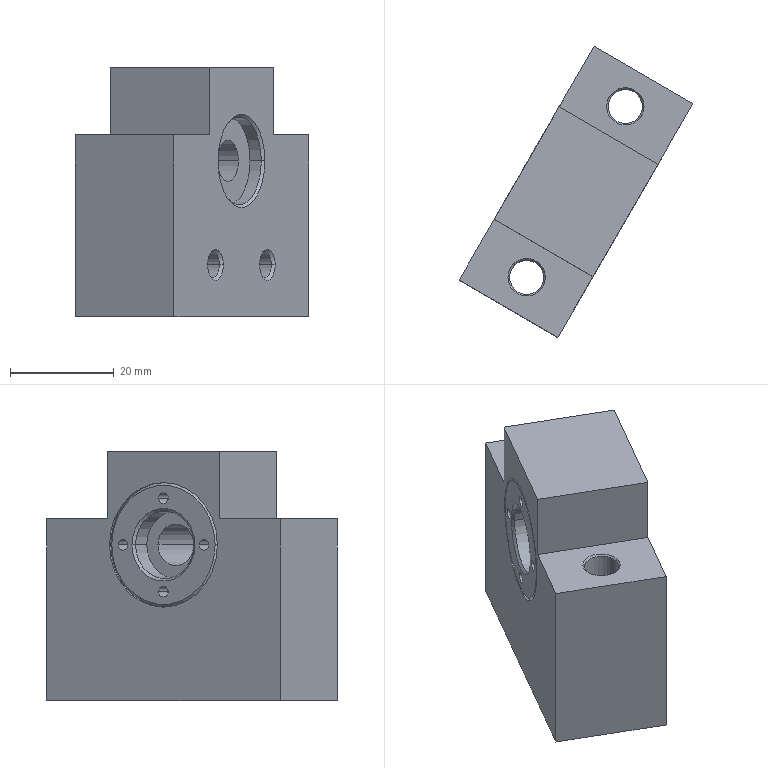Part | SolidWorks | features BaseBody 1 | 1 solid | 59 faces | box 45.053 x 56.033 x 48 mm | volume 42155 mm3 | cylinder 24 | cone 18 | plane 17 | commonest cylinder face diameters 2.1 x8 4.917 x4 6.6 x4 8 x2 13 x2 17 x2